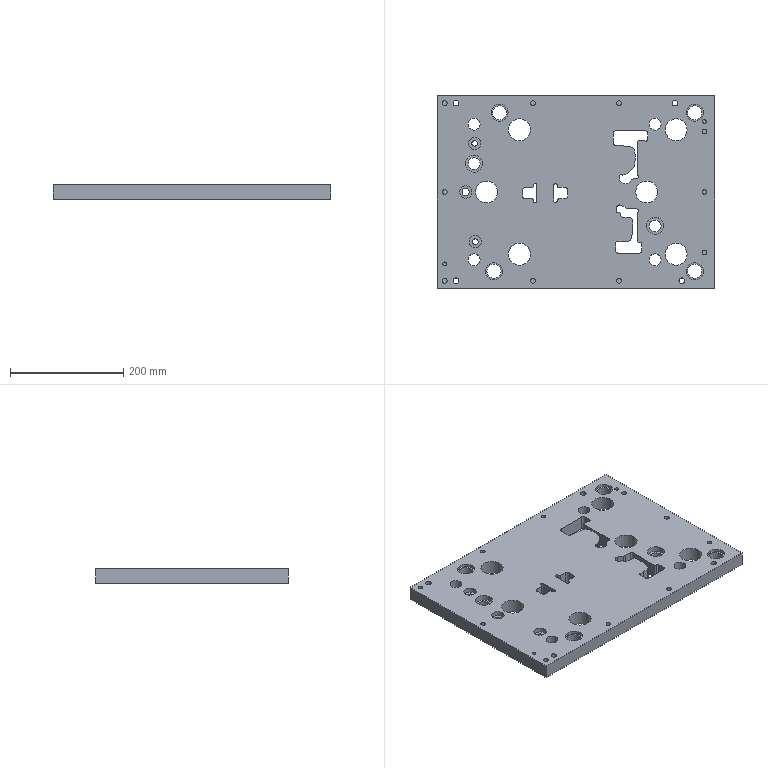Part | NX | features LIN_SOLID_COLOR 2 | 1 solid | 177 faces | box 490 x 340 x 25 mm | volume 3702689 mm3 | cylinder 88 | plane 87 | cone 2 | commonest cylinder face diameters 6 x20 8.5 x10 10 x10 4 x6 21 x6 30 x6